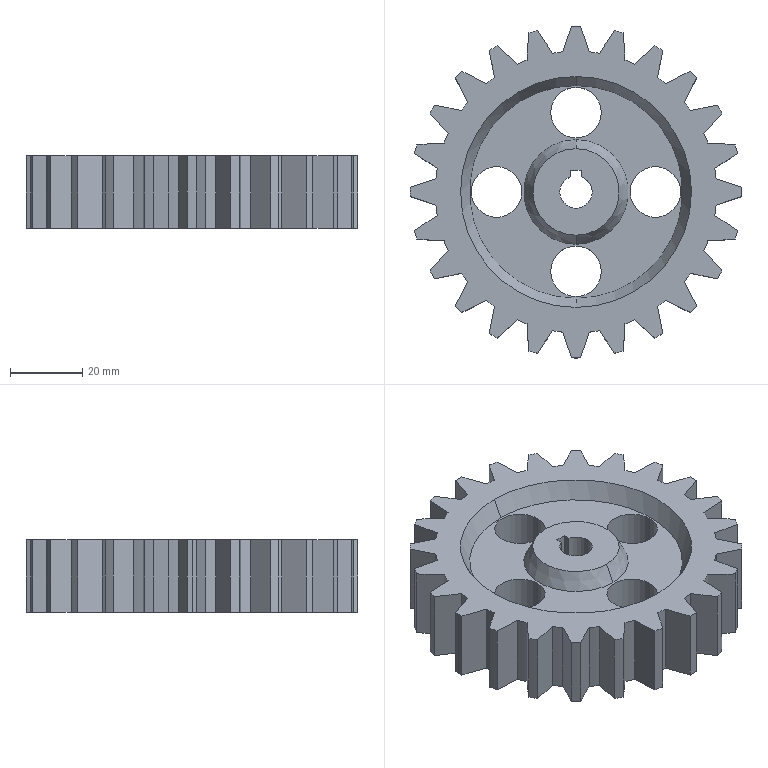Part | NX | features BREP 1 | 1 solid | 125 faces | box 92 x 92 x 20 mm | volume 80350 mm3 | cylinder 60 | plane 57 | cone 8 | commonest cylinder face diameters 92 x25 78 x24 14 x8 9 x3